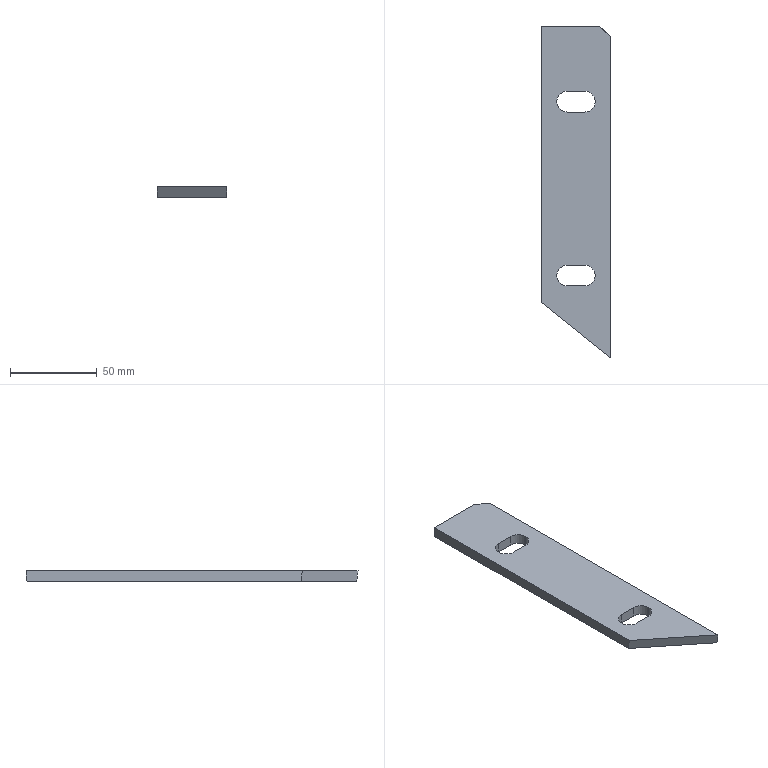Part | STEP file | 粉仓楼梯护栏连接Plate | 1 solid | 17 faces | box 40 x 190.865 x 6 mm | volume 38885 mm3 | plane 11 | cylinder 6 | commonest cylinder face diameters 12 x6
STEP:
#1=CARTESIAN_POINT('',(0.,0.,0.));
#2=DIRECTION('',(0.,0.,1.));
#3=DIRECTION('',(1.,0.,0.));
#4=AXIS2_PLACEMENT_3D('',#1,#2,#3);
#5=CARTESIAN_POINT('',(5.,56.,0.));
#6=VERTEX_POINT('',#5);
#7=CARTESIAN_POINT('',(5.,56.,6.));
#8=VERTEX_POINT('',#7);
#9=CARTESIAN_POINT('',(5.,56.,6.));
#10=DIRECTION('',(0.,0.,1.));
#11=VECTOR('',#10,1.);
#12=LINE('',#9,#11);
#13=CARTESIAN_POINT('',(5.,50.,6.));
#14=DIRECTION('',(0.,0.,1.));
#15=DIRECTION('',(1.,0.,0.));
#16=AXIS2_PLACEMENT_3D('',#13,#14,#15);
#17=CYLINDRICAL_SURFACE('',#16,6.);
#18=CARTESIAN_POINT('',(1.571,0.));
#19=DIRECTION('',(0.,1.));
#20=VECTOR('',#19,1.);
#21=LINE('',#18,#20);
#22=(GEOMETRIC_REPRESENTATION_CONTEXT(2)PARAMETRIC_REPRESENTATION_CONTEXT()REPRESENTATION_CONTEXT('',''));
#23=DEFINITIONAL_REPRESENTATION('',(#21),#22);
#24=PCURVE('',#17,#23);
#25=CARTESIAN_POINT('',(-5.,56.,6.));
#26=DIRECTION('',(0.,1.,0.));
#27=DIRECTION('',(0.,0.,1.));
#28=AXIS2_PLACEMENT_3D('',#25,#26,#27);
#29=PLANE('',#28);
#30=CARTESIAN_POINT('',(0.,10.));
#31=DIRECTION('',(1.,0.));
#32=VECTOR('',#31,1.);
#33=LINE('',#30,#32);
#34=(GEOMETRIC_REPRESENTATION_CONTEXT(2)PARAMETRIC_REPRESENTATION_CONTEXT()REPRESENTATION_CONTEXT('',''));
#35=DEFINITIONAL_REPRESENTATION('',(#33),#34);
#36=PCURVE('',#29,#35);
#37=SURFACE_CURVE('',#12,(#24,#36),.PCURVE_S1.);
#38=EDGE_CURVE('',#6,#8,#37,.T.);
#39=ORIENTED_EDGE('',*,*,#38,.T.);
#40=CARTESIAN_POINT('',(11.,50.,6.));
#41=VERTEX_POINT('',#40);
#42=CARTESIAN_POINT('',(5.,50.,6.));
#43=DIRECTION('',(0.,0.,1.));
#44=DIRECTION('',(1.,0.,0.));
#45=AXIS2_PLACEMENT_3D('',#42,#43,#44);
#46=CIRCLE('',#45,6.);
#47=CARTESIAN_POINT('',(0.,0.));
#48=DIRECTION('',(1.,0.));
#49=VECTOR('',#48,1.);
#50=LINE('',#47,#49);
#51=(GEOMETRIC_REPRESENTATION_CONTEXT(2)PARAMETRIC_REPRESENTATION_CONTEXT()REPRESENTATION_CONTEXT('',''));
#52=DEFINITIONAL_REPRESENTATION('',(#50),#51);
#53=PCURVE('',#17,#52);
#54=CARTESIAN_POINT('',(0.,0.,6.));
#55=DIRECTION('',(0.,0.,1.));
#56=DIRECTION('',(1.,0.,0.));
#57=AXIS2_PLACEMENT_3D('',#54,#55,#56);
#58=PLANE('',#57);
#59=CARTESIAN_POINT('',(5.,50.));
#60=DIRECTION('',(1.,0.));
#61=AXIS2_PLACEMENT_2D('',#59,#60);
#62=CIRCLE('',#61,6.);
#63=(GEOMETRIC_REPRESENTATION_CONTEXT(2)PARAMETRIC_REPRESENTATION_CONTEXT()REPRESENTATION_CONTEXT('',''));
#64=DEFINITIONAL_REPRESENTATION('',(#62),#63);
#65=PCURVE('',#58,#64);
#66=SURFACE_CURVE('',#46,(#53,#65),.PCURVE_S1.);
#67=EDGE_CURVE('',#41,#8,#66,.T.);
#68=ORIENTED_EDGE('',*,*,#67,.F.);
#69=CARTESIAN_POINT('',(11.,50.,0.));
#70=VERTEX_POINT('',#69);
#71=CARTESIAN_POINT('',(11.,50.,6.));
#72=DIRECTION('',(0.,0.,1.));
#73=VECTOR('',#72,1.);
#74=LINE('',#71,#73);
#75=CARTESIAN_POINT('',(0.,0.));
#76=DIRECTION('',(0.,1.));
#77=VECTOR('',#76,1.);
#78=LINE('',#75,#77);
#79=(GEOMETRIC_REPRESENTATION_CONTEXT(2)PARAMETRIC_REPRESENTATION_CONTEXT()REPRESENTATION_CONTEXT('',''));
#80=DEFINITIONAL_REPRESENTATION('',(#78),#79);
#81=PCURVE('',#17,#80);
#82=CARTESIAN_POINT('',(5.,50.,6.));
#83=DIRECTION('',(0.,0.,1.));
#84=DIRECTION('',(1.,0.,0.));
#85=AXIS2_PLACEMENT_3D('',#82,#83,#84);
#86=CYLINDRICAL_SURFACE('',#85,6.);
#87=CARTESIAN_POINT('',(6.283,0.));
#88=DIRECTION('',(0.,1.));
#89=VECTOR('',#88,1.);
#90=LINE('',#87,#89);
#91=(GEOMETRIC_REPRESENTATION_CONTEXT(2)PARAMETRIC_REPRESENTATION_CONTEXT()REPRESENTATION_CONTEXT('',''));
#92=DEFINITIONAL_REPRESENTATION('',(#90),#91);
#93=PCURVE('',#86,#92);
#94=SURFACE_CURVE('',#74,(#81,#93),.PCURVE_S1.);
#95=EDGE_CURVE('',#70,#41,#94,.T.);
#96=ORIENTED_EDGE('',*,*,#95,.F.);
#97=CARTESIAN_POINT('',(5.,50.,0.));
#98=DIRECTION('',(0.,0.,1.));
#99=DIRECTION('',(1.,0.,0.));
#100=AXIS2_PLACEMENT_3D('',#97,#98,#99);
#101=CIRCLE('',#100,6.);
#102=CARTESIAN_POINT('',(0.,-6.));
#103=DIRECTION('',(1.,0.));
#104=VECTOR('',#103,1.);
#105=LINE('',#102,#104);
#106=(GEOMETRIC_REPRESENTATION_CONTEXT(2)PARAMETRIC_REPRESENTATION_CONTEXT()REPRESENTATION_CONTEXT('',''));
#107=DEFINITIONAL_REPRESENTATION('',(#105),#106);
#108=PCURVE('',#17,#107);
#109=CARTESIAN_POINT('',(0.,0.,0.));
#110=DIRECTION('',(0.,0.,1.));
#111=DIRECTION('',(1.,0.,0.));
#112=AXIS2_PLACEMENT_3D('',#109,#110,#111);
#113=PLANE('',#112);
#114=CARTESIAN_POINT('',(5.,50.));
#115=DIRECTION('',(1.,0.));
#116=AXIS2_PLACEMENT_2D('',#114,#115);
#117=CIRCLE('',#116,6.);
#118=(GEOMETRIC_REPRESENTATION_CONTEXT(2)PARAMETRIC_REPRESENTATION_CONTEXT()REPRESENTATION_CONTEXT('',''));
#119=DEFINITIONAL_REPRESENTATION('',(#117),#118);
#120=PCURVE('',#113,#119);
#121=SURFACE_CURVE('',#101,(#108,#120),.PCURVE_S1.);
#122=EDGE_CURVE('',#70,#6,#121,.T.);
#123=ORIENTED_EDGE('',*,*,#122,.T.);
#124=EDGE_LOOP('',(#39,#68,#96,#123));
#125=FACE_BOUND('',#124,.F.);
#126=ADVANCED_FACE('',(#125),#17,.F.);
#127=CARTESIAN_POINT('',(5.,-44.,0.));
#128=VERTEX_POINT('',#127);
#129=CARTESIAN_POINT('',(5.,-44.,6.));
#130=VERTEX_POINT('',#129);
#131=CARTESIAN_POINT('',(5.,-44.,6.));
#132=DIRECTION('',(0.,0.,1.));
#133=VECTOR('',#132,1.);
#134=LINE('',#131,#133);
#135=CARTESIAN_POINT('',(5.,-50.,6.));
#136=DIRECTION('',(0.,0.,1.));
#137=DIRECTION('',(1.,0.,0.));
#138=AXIS2_PLACEMENT_3D('',#135,#136,#137);
#139=CYLINDRICAL_SURFACE('',#138,6.);
#140=CARTESIAN_POINT('',(1.571,0.));
#141=DIRECTION('',(0.,1.));
#142=VECTOR('',#141,1.);
#143=LINE('',#140,#142);
#144=(GEOMETRIC_REPRESENTATION_CONTEXT(2)PARAMETRIC_REPRESENTATION_CONTEXT()REPRESENTATION_CONTEXT('',''));
#145=DEFINITIONAL_REPRESENTATION('',(#143),#144);
#146=PCURVE('',#139,#145);
#147=CARTESIAN_POINT('',(-5.,-44.,6.));
#148=DIRECTION('',(0.,1.,0.));
#149=DIRECTION('',(0.,0.,1.));
#150=AXIS2_PLACEMENT_3D('',#147,#148,#149);
#151=PLANE('',#150);
#152=CARTESIAN_POINT('',(0.,10.));
#153=DIRECTION('',(1.,0.));
#154=VECTOR('',#153,1.);
#155=LINE('',#152,#154);
#156=(GEOMETRIC_REPRESENTATION_CONTEXT(2)PARAMETRIC_REPRESENTATION_CONTEXT()REPRESENTATION_CONTEXT('',''));
#157=DEFINITIONAL_REPRESENTATION('',(#155),#156);
#158=PCURVE('',#151,#157);
#159=SURFACE_CURVE('',#134,(#146,#158),.PCURVE_S1.);
#160=EDGE_CURVE('',#128,#130,#159,.T.);
#161=ORIENTED_EDGE('',*,*,#160,.T.);
#162=CARTESIAN_POINT('',(11.,-50.,6.));
#163=VERTEX_POINT('',#162);
#164=CARTESIAN_POINT('',(5.,-50.,6.));
#165=DIRECTION('',(0.,0.,1.));
#166=DIRECTION('',(1.,0.,0.));
#167=AXIS2_PLACEMENT_3D('',#164,#165,#166);
#168=CIRCLE('',#167,6.);
#169=CARTESIAN_POINT('',(0.,0.));
#170=DIRECTION('',(1.,0.));
#171=VECTOR('',#170,1.);
#172=LINE('',#169,#171);
#173=(GEOMETRIC_REPRESENTATION_CONTEXT(2)PARAMETRIC_REPRESENTATION_CONTEXT()REPRESENTATION_CONTEXT('',''));
#174=DEFINITIONAL_REPRESENTATION('',(#172),#173);
#175=PCURVE('',#139,#174);
#176=CARTESIAN_POINT('',(5.,-50.));
#177=DIRECTION('',(1.,0.));
#178=AXIS2_PLACEMENT_2D('',#176,#177);
#179=CIRCLE('',#178,6.);
#180=(GEOMETRIC_REPRESENTATION_CONTEXT(2)PARAMETRIC_REPRESENTATION_CONTEXT()REPRESENTATION_CONTEXT('',''));
#181=DEFINITIONAL_REPRESENTATION('',(#179),#180);
#182=PCURVE('',#58,#181);
#183=SURFACE_CURVE('',#168,(#175,#182),.PCURVE_S1.);
#184=EDGE_CURVE('',#163,#130,#183,.T.);
#185=ORIENTED_EDGE('',*,*,#184,.F.);
#186=CARTESIAN_POINT('',(11.,-50.,0.));
#187=VERTEX_POINT('',#186);
#188=CARTESIAN_POINT('',(11.,-50.,6.));
#189=DIRECTION('',(0.,0.,1.));
#190=VECTOR('',#189,1.);
#191=LINE('',#188,#190);
#192=CARTESIAN_POINT('',(0.,0.));
#193=DIRECTION('',(0.,1.));
#194=VECTOR('',#193,1.);
#195=LINE('',#192,#194);
#196=(GEOMETRIC_REPRESENTATION_CONTEXT(2)PARAMETRIC_REPRESENTATION_CONTEXT()REPRESENTATION_CONTEXT('',''));
#197=DEFINITIONAL_REPRESENTATION('',(#195),#196);
#198=PCURVE('',#139,#197);
#199=CARTESIAN_POINT('',(5.,-50.,6.));
#200=DIRECTION('',(0.,0.,1.));
#201=DIRECTION('',(1.,0.,0.));
#202=AXIS2_PLACEMENT_3D('',#199,#200,#201);
#203=CYLINDRICAL_SURFACE('',#202,6.);
#204=CARTESIAN_POINT('',(6.283,0.));
#205=DIRECTION('',(0.,1.));
#206=VECTOR('',#205,1.);
#207=LINE('',#204,#206);
#208=(GEOMETRIC_REPRESENTATION_CONTEXT(2)PARAMETRIC_REPRESENTATION_CONTEXT()REPRESENTATION_CONTEXT('',''));
#209=DEFINITIONAL_REPRESENTATION('',(#207),#208);
#210=PCURVE('',#203,#209);
#211=SURFACE_CURVE('',#191,(#198,#210),.PCURVE_S1.);
#212=EDGE_CURVE('',#187,#163,#211,.T.);
#213=ORIENTED_EDGE('',*,*,#212,.F.);
#214=CARTESIAN_POINT('',(5.,-50.,0.));
#215=DIRECTION('',(0.,0.,1.));
#216=DIRECTION('',(1.,0.,0.));
#217=AXIS2_PLACEMENT_3D('',#214,#215,#216);
#218=CIRCLE('',#217,6.);
#219=CARTESIAN_POINT('',(0.,-6.));
#220=DIRECTION('',(1.,0.));
#221=VECTOR('',#220,1.);
#222=LINE('',#219,#221);
#223=(GEOMETRIC_REPRESENTATION_CONTEXT(2)PARAMETRIC_REPRESENTATION_CONTEXT()REPRESENTATION_CONTEXT('',''));
#224=DEFINITIONAL_REPRESENTATION('',(#222),#223);
#225=PCURVE('',#139,#224);
#226=CARTESIAN_POINT('',(5.,-50.));
#227=DIRECTION('',(1.,0.));
#228=AXIS2_PLACEMENT_2D('',#226,#227);
#229=CIRCLE('',#228,6.);
#230=(GEOMETRIC_REPRESENTATION_CONTEXT(2)PARAMETRIC_REPRESENTATION_CONTEXT()REPRESENTATION_CONTEXT('',''));
#231=DEFINITIONAL_REPRESENTATION('',(#229),#230);
#232=PCURVE('',#113,#231);
#233=SURFACE_CURVE('',#218,(#225,#232),.PCURVE_S1.);
#234=EDGE_CURVE('',#187,#128,#233,.T.);
#235=ORIENTED_EDGE('',*,*,#234,.T.);
#236=EDGE_LOOP('',(#161,#185,#213,#235));
#237=FACE_BOUND('',#236,.F.);
#238=ADVANCED_FACE('',(#237),#139,.F.);
#239=CARTESIAN_POINT('',(20.,-96.589,0.));
#240=VERTEX_POINT('',#239);
#241=CARTESIAN_POINT('',(20.,87.469,0.));
#242=VERTEX_POINT('',#241);
#243=CARTESIAN_POINT('',(20.,92.,0.));
#244=DIRECTION('',(0.,1.,0.));
#245=VECTOR('',#244,1.);
#246=LINE('',#243,#245);
#247=CARTESIAN_POINT('',(20.,92.,6.));
#248=DIRECTION('',(-1.,0.,0.));
#249=DIRECTION('',(0.,-1.,0.));
#250=AXIS2_PLACEMENT_3D('',#247,#248,#249);
#251=PLANE('',#250);
#252=CARTESIAN_POINT('',(0.,-6.));
#253=DIRECTION('',(-1.,0.));
#254=VECTOR('',#253,1.);
#255=LINE('',#252,#254);
#256=(GEOMETRIC_REPRESENTATION_CONTEXT(2)PARAMETRIC_REPRESENTATION_CONTEXT()REPRESENTATION_CONTEXT('',''));
#257=DEFINITIONAL_REPRESENTATION('',(#255),#256);
#258=PCURVE('',#251,#257);
#259=CARTESIAN_POINT('',(20.,92.));
#260=DIRECTION('',(0.,1.));
#261=VECTOR('',#260,1.);
#262=LINE('',#259,#261);
#263=(GEOMETRIC_REPRESENTATION_CONTEXT(2)PARAMETRIC_REPRESENTATION_CONTEXT()REPRESENTATION_CONTEXT('',''));
#264=DEFINITIONAL_REPRESENTATION('',(#262),#263);
#265=PCURVE('',#113,#264);
#266=SURFACE_CURVE('',#246,(#258,#265),.PCURVE_S1.);
#267=EDGE_CURVE('',#240,#242,#266,.T.);
#268=ORIENTED_EDGE('',*,*,#267,.T.);
#269=CARTESIAN_POINT('',(20.,87.469,6.));
#270=VERTEX_POINT('',#269);
#271=CARTESIAN_POINT('',(20.,87.469,0.));
#272=DIRECTION('',(0.,0.,1.));
#273=VECTOR('',#272,1.);
#274=LINE('',#271,#273);
#275=CARTESIAN_POINT('',(4.531,-6.));
#276=DIRECTION('',(0.,1.));
#277=VECTOR('',#276,1.);
#278=LINE('',#275,#277);
#279=(GEOMETRIC_REPRESENTATION_CONTEXT(2)PARAMETRIC_REPRESENTATION_CONTEXT()REPRESENTATION_CONTEXT('',''));
#280=DEFINITIONAL_REPRESENTATION('',(#278),#279);
#281=PCURVE('',#251,#280);
#282=CARTESIAN_POINT('',(20.,87.469,0.));
#283=DIRECTION('',(-0.6508,-0.7593,0.));
#284=DIRECTION('',(0.7593,-0.6508,0.));
#285=AXIS2_PLACEMENT_3D('',#282,#283,#284);
#286=PLANE('',#285);
#287=CARTESIAN_POINT('',(0.,0.));
#288=DIRECTION('',(0.,1.));
#289=VECTOR('',#288,1.);
#290=LINE('',#287,#289);
#291=(GEOMETRIC_REPRESENTATION_CONTEXT(2)PARAMETRIC_REPRESENTATION_CONTEXT()REPRESENTATION_CONTEXT('',''));
#292=DEFINITIONAL_REPRESENTATION('',(#290),#291);
#293=PCURVE('',#286,#292);
#294=SURFACE_CURVE('',#274,(#281,#293),.PCURVE_S1.);
#295=EDGE_CURVE('',#242,#270,#294,.T.);
#296=ORIENTED_EDGE('',*,*,#295,.T.);
#297=CARTESIAN_POINT('',(20.,-97.396,6.));
#298=VERTEX_POINT('',#297);
#299=CARTESIAN_POINT('',(20.,92.,6.));
#300=DIRECTION('',(0.,1.,0.));
#301=VECTOR('',#300,1.);
#302=LINE('',#299,#301);
#303=CARTESIAN_POINT('',(0.,0.));
#304=DIRECTION('',(-1.,0.));
#305=VECTOR('',#304,1.);
#306=LINE('',#303,#305);
#307=(GEOMETRIC_REPRESENTATION_CONTEXT(2)PARAMETRIC_REPRESENTATION_CONTEXT()REPRESENTATION_CONTEXT('',''));
#308=DEFINITIONAL_REPRESENTATION('',(#306),#307);
#309=PCURVE('',#251,#308);
#310=CARTESIAN_POINT('',(20.,92.));
#311=DIRECTION('',(0.,1.));
#312=VECTOR('',#311,1.);
#313=LINE('',#310,#312);
#314=(GEOMETRIC_REPRESENTATION_CONTEXT(2)PARAMETRIC_REPRESENTATION_CONTEXT()REPRESENTATION_CONTEXT('',''));
#315=DEFINITIONAL_REPRESENTATION('',(#313),#314);
#316=PCURVE('',#58,#315);
#317=SURFACE_CURVE('',#302,(#309,#316),.PCURVE_S1.);
#318=EDGE_CURVE('',#298,#270,#317,.T.);
#319=ORIENTED_EDGE('',*,*,#318,.F.);
#320=CARTESIAN_POINT('',(20.,-97.134,4.055));
#321=DIRECTION('',(0.,-0.1334,0.9911));
#322=VECTOR('',#321,1.);
#323=LINE('',#320,#322);
#324=CARTESIAN_POINT('',(189.134,-1.945));
#325=DIRECTION('',(0.1334,0.9911));
#326=VECTOR('',#325,1.);
#327=LINE('',#324,#326);
#328=(GEOMETRIC_REPRESENTATION_CONTEXT(2)PARAMETRIC_REPRESENTATION_CONTEXT()REPRESENTATION_CONTEXT('',''));
#329=DEFINITIONAL_REPRESENTATION('',(#327),#328);
#330=PCURVE('',#251,#329);
#331=CARTESIAN_POINT('',(2925.063,-2415.047,-41.545));
#332=DIRECTION('',(-0.6213,-0.7766,-0.1045));
#333=DIRECTION('',(0.7809,-0.6247,0.));
#334=AXIS2_PLACEMENT_3D('',#331,#332,#333);
#335=PLANE('',#334);
#336=CARTESIAN_POINT('',(-3716.461,45.851));
#337=DIRECTION('',(0.08333,0.9965));
#338=VECTOR('',#337,1.);
#339=LINE('',#336,#338);
#340=(GEOMETRIC_REPRESENTATION_CONTEXT(2)PARAMETRIC_REPRESENTATION_CONTEXT()REPRESENTATION_CONTEXT('',''));
#341=DEFINITIONAL_REPRESENTATION('',(#339),#340);
#342=PCURVE('',#335,#341);
#343=SURFACE_CURVE('',#323,(#330,#342),.PCURVE_S1.);
#344=EDGE_CURVE('',#240,#298,#343,.T.);
#345=ORIENTED_EDGE('',*,*,#344,.F.);
#346=EDGE_LOOP('',(#268,#296,#319,#345));
#347=FACE_BOUND('',#346,.T.);
#348=ADVANCED_FACE('',(#347),#251,.F.);
#349=CARTESIAN_POINT('',(-20.,92.839,0.));
#350=VERTEX_POINT('',#349);
#351=CARTESIAN_POINT('',(-20.,-64.589,0.));
#352=VERTEX_POINT('',#351);
#353=CARTESIAN_POINT('',(-20.,92.,0.));
#354=DIRECTION('',(0.,-1.,0.));
#355=VECTOR('',#354,1.);
#356=LINE('',#353,#355);
#357=CARTESIAN_POINT('',(-20.,92.,6.));
#358=DIRECTION('',(1.,0.,0.));
#359=DIRECTION('',(0.,1.,0.));
#360=AXIS2_PLACEMENT_3D('',#357,#358,#359);
#361=PLANE('',#360);
#362=CARTESIAN_POINT('',(0.,-6.));
#363=DIRECTION('',(-1.,0.));
#364=VECTOR('',#363,1.);
#365=LINE('',#362,#364);
#366=(GEOMETRIC_REPRESENTATION_CONTEXT(2)PARAMETRIC_REPRESENTATION_CONTEXT()REPRESENTATION_CONTEXT('',''));
#367=DEFINITIONAL_REPRESENTATION('',(#365),#366);
#368=PCURVE('',#361,#367);
#369=CARTESIAN_POINT('',(-20.,92.));
#370=DIRECTION('',(0.,-1.));
#371=VECTOR('',#370,1.);
#372=LINE('',#369,#371);
#373=(GEOMETRIC_REPRESENTATION_CONTEXT(2)PARAMETRIC_REPRESENTATION_CONTEXT()REPRESENTATION_CONTEXT('',''));
#374=DEFINITIONAL_REPRESENTATION('',(#372),#373);
#375=PCURVE('',#113,#374);
#376=SURFACE_CURVE('',#356,(#368,#375),.PCURVE_S1.);
#377=EDGE_CURVE('',#350,#352,#376,.T.);
#378=ORIENTED_EDGE('',*,*,#377,.T.);
#379=CARTESIAN_POINT('',(-20.,-65.396,6.));
#380=VERTEX_POINT('',#379);
#381=CARTESIAN_POINT('',(-20.,-66.497,14.178));
#382=DIRECTION('',(0.,0.1334,-0.9911));
#383=VECTOR('',#382,1.);
#384=LINE('',#381,#383);
#385=CARTESIAN_POINT('',(-158.497,8.178));
#386=DIRECTION('',(0.1334,-0.9911));
#387=VECTOR('',#386,1.);
#388=LINE('',#385,#387);
#389=(GEOMETRIC_REPRESENTATION_CONTEXT(2)PARAMETRIC_REPRESENTATION_CONTEXT()REPRESENTATION_CONTEXT('',''));
#390=DEFINITIONAL_REPRESENTATION('',(#388),#389);
#391=PCURVE('',#361,#390);
#392=CARTESIAN_POINT('',(-3766.835,56.031));
#393=DIRECTION('',(-0.08333,-0.9965));
#394=VECTOR('',#393,1.);
#395=LINE('',#392,#394);
#396=(GEOMETRIC_REPRESENTATION_CONTEXT(2)PARAMETRIC_REPRESENTATION_CONTEXT()REPRESENTATION_CONTEXT('',''));
#397=DEFINITIONAL_REPRESENTATION('',(#395),#396);
#398=PCURVE('',#335,#397);
#399=SURFACE_CURVE('',#384,(#391,#398),.PCURVE_S1.);
#400=EDGE_CURVE('',#380,#352,#399,.T.);
#401=ORIENTED_EDGE('',*,*,#400,.F.);
#402=CARTESIAN_POINT('',(-20.,93.469,6.));
#403=VERTEX_POINT('',#402);
#404=CARTESIAN_POINT('',(-20.,92.,6.));
#405=DIRECTION('',(0.,-1.,0.));
#406=VECTOR('',#405,1.);
#407=LINE('',#404,#406);
#408=CARTESIAN_POINT('',(0.,0.));
#409=DIRECTION('',(-1.,0.));
#410=VECTOR('',#409,1.);
#411=LINE('',#408,#410);
#412=(GEOMETRIC_REPRESENTATION_CONTEXT(2)PARAMETRIC_REPRESENTATION_CONTEXT()REPRESENTATION_CONTEXT('',''));
#413=DEFINITIONAL_REPRESENTATION('',(#411),#412);
#414=PCURVE('',#361,#413);
#415=CARTESIAN_POINT('',(-20.,92.));
#416=DIRECTION('',(0.,-1.));
#417=VECTOR('',#416,1.);
#418=LINE('',#415,#417);
#419=(GEOMETRIC_REPRESENTATION_CONTEXT(2)PARAMETRIC_REPRESENTATION_CONTEXT()REPRESENTATION_CONTEXT('',''));
#420=DEFINITIONAL_REPRESENTATION('',(#418),#419);
#421=PCURVE('',#58,#420);
#422=SURFACE_CURVE('',#407,(#414,#421),.PCURVE_S1.);
#423=EDGE_CURVE('',#403,#380,#422,.T.);
#424=ORIENTED_EDGE('',*,*,#423,.F.);
#425=CARTESIAN_POINT('',(-20.,93.285,4.249));
#426=DIRECTION('',(0.,0.1045,0.9945));
#427=VECTOR('',#426,1.);
#428=LINE('',#425,#427);
#429=CARTESIAN_POINT('',(1.285,-1.751));
#430=DIRECTION('',(0.1045,0.9945));
#431=VECTOR('',#430,1.);
#432=LINE('',#429,#431);
#433=(GEOMETRIC_REPRESENTATION_CONTEXT(2)PARAMETRIC_REPRESENTATION_CONTEXT()REPRESENTATION_CONTEXT('',''));
#434=DEFINITIONAL_REPRESENTATION('',(#432),#433);
#435=PCURVE('',#361,#434);
#436=CARTESIAN_POINT('',(17.5,88.472,-41.545));
#437=DIRECTION('',(0.,0.9945,-0.1045));
#438=DIRECTION('',(0.,-0.1045,-0.9945));
#439=AXIS2_PLACEMENT_3D('',#436,#437,#438);
#440=PLANE('',#439);
#441=CARTESIAN_POINT('',(-46.047,37.5));
#442=DIRECTION('',(-1.,0.));
#443=VECTOR('',#442,1.);
#444=LINE('',#441,#443);
#445=(GEOMETRIC_REPRESENTATION_CONTEXT(2)PARAMETRIC_REPRESENTATION_CONTEXT()REPRESENTATION_CONTEXT('',''));
#446=DEFINITIONAL_REPRESENTATION('',(#444),#445);
#447=PCURVE('',#440,#446);
#448=SURFACE_CURVE('',#428,(#435,#447),.PCURVE_S1.);
#449=EDGE_CURVE('',#350,#403,#448,.T.);
#450=ORIENTED_EDGE('',*,*,#449,.F.);
#451=EDGE_LOOP('',(#378,#401,#424,#450));
#452=FACE_BOUND('',#451,.T.);
#453=ADVANCED_FACE('',(#452),#361,.F.);
#454=CARTESIAN_POINT('',(13.,93.469,6.));
#455=VERTEX_POINT('',#454);
#456=CARTESIAN_POINT('',(20.,87.469,6.));
#457=DIRECTION('',(0.7593,-0.6508,0.));
#458=VECTOR('',#457,1.);
#459=LINE('',#456,#458);
#460=CARTESIAN_POINT('',(20.,87.469));
#461=DIRECTION('',(0.7593,-0.6508));
#462=VECTOR('',#461,1.);
#463=LINE('',#460,#462);
#464=(GEOMETRIC_REPRESENTATION_CONTEXT(2)PARAMETRIC_REPRESENTATION_CONTEXT()REPRESENTATION_CONTEXT('',''));
#465=DEFINITIONAL_REPRESENTATION('',(#463),#464);
#466=PCURVE('',#58,#465);
#467=CARTESIAN_POINT('',(0.,6.));
#468=DIRECTION('',(1.,0.));
#469=VECTOR('',#468,1.);
#470=LINE('',#467,#469);
#471=(GEOMETRIC_REPRESENTATION_CONTEXT(2)PARAMETRIC_REPRESENTATION_CONTEXT()REPRESENTATION_CONTEXT('',''));
#472=DEFINITIONAL_REPRESENTATION('',(#470),#471);
#473=PCURVE('',#286,#472);
#474=SURFACE_CURVE('',#459,(#466,#473),.PCURVE_S1.);
#475=EDGE_CURVE('',#455,#270,#474,.T.);
#476=ORIENTED_EDGE('',*,*,#475,.F.);
#477=CARTESIAN_POINT('',(-20.,93.469,6.));
#478=DIRECTION('',(1.,0.,0.));
#479=VECTOR('',#478,1.);
#480=LINE('',#477,#479);
#481=CARTESIAN_POINT('',(-20.,93.469));
#482=DIRECTION('',(1.,0.));
#483=VECTOR('',#482,1.);
#484=LINE('',#481,#483);
#485=(GEOMETRIC_REPRESENTATION_CONTEXT(2)PARAMETRIC_REPRESENTATION_CONTEXT()REPRESENTATION_CONTEXT('',''));
#486=DEFINITIONAL_REPRESENTATION('',(#484),#485);
#487=PCURVE('',#58,#486);
#488=CARTESIAN_POINT('',(-47.807,37.5));
#489=DIRECTION('',(0.,-1.));
#490=VECTOR('',#489,1.);
#491=LINE('',#488,#490);
#492=(GEOMETRIC_REPRESENTATION_CONTEXT(2)PARAMETRIC_REPRESENTATION_CONTEXT()REPRESENTATION_CONTEXT('',''));
#493=DEFINITIONAL_REPRESENTATION('',(#491),#492);
#494=PCURVE('',#440,#493);
#495=SURFACE_CURVE('',#480,(#487,#494),.PCURVE_S1.);
#496=EDGE_CURVE('',#403,#455,#495,.T.);
#497=ORIENTED_EDGE('',*,*,#496,.F.);
#498=ORIENTED_EDGE('',*,*,#423,.T.);
#499=CARTESIAN_POINT('',(34.567,-109.049,6.));
#500=DIRECTION('',(-0.7809,0.6247,0.));
#501=VECTOR('',#500,1.);
#502=LINE('',#499,#501);
#503=CARTESIAN_POINT('',(34.567,-109.049));
#504=DIRECTION('',(-0.7809,0.6247));
#505=VECTOR('',#504,1.);
#506=LINE('',#503,#505);
#507=(GEOMETRIC_REPRESENTATION_CONTEXT(2)PARAMETRIC_REPRESENTATION_CONTEXT()REPRESENTATION_CONTEXT('',''));
#508=DEFINITIONAL_REPRESENTATION('',(#506),#507);
#509=PCURVE('',#58,#508);
#510=CARTESIAN_POINT('',(-3697.643,47.807));
#511=DIRECTION('',(-1.,0.));
#512=VECTOR('',#511,1.);
#513=LINE('',#510,#512);
#514=(GEOMETRIC_REPRESENTATION_CONTEXT(2)PARAMETRIC_REPRESENTATION_CONTEXT()REPRESENTATION_CONTEXT('',''));
#515=DEFINITIONAL_REPRESENTATION('',(#513),#514);
#516=PCURVE('',#335,#515);
#517=SURFACE_CURVE('',#502,(#509,#516),.PCURVE_S1.);
#518=EDGE_CURVE('',#298,#380,#517,.T.);
#519=ORIENTED_EDGE('',*,*,#518,.F.);
#520=ORIENTED_EDGE('',*,*,#318,.T.);
#521=EDGE_LOOP('',(#476,#497,#498,#519,#520));
#522=FACE_BOUND('',#521,.T.);
#523=CARTESIAN_POINT('',(-5.,44.,6.));
#524=VERTEX_POINT('',#523);
#525=CARTESIAN_POINT('',(5.,44.,6.));
#526=VERTEX_POINT('',#525);
#527=CARTESIAN_POINT('',(-5.,44.,6.));
#528=DIRECTION('',(1.,0.,0.));
#529=VECTOR('',#528,1.);
#530=LINE('',#527,#529);
#531=CARTESIAN_POINT('',(-5.,44.));
#532=DIRECTION('',(1.,0.));
#533=VECTOR('',#532,1.);
#534=LINE('',#531,#533);
#535=(GEOMETRIC_REPRESENTATION_CONTEXT(2)PARAMETRIC_REPRESENTATION_CONTEXT()REPRESENTATION_CONTEXT('',''));
#536=DEFINITIONAL_REPRESENTATION('',(#534),#535);
#537=PCURVE('',#58,#536);
#538=CARTESIAN_POINT('',(-5.,44.,6.));
#539=DIRECTION('',(0.,-1.,0.));
#540=DIRECTION('',(0.,0.,-1.));
#541=AXIS2_PLACEMENT_3D('',#538,#539,#540);
#542=PLANE('',#541);
#543=CARTESIAN_POINT('',(0.,0.));
#544=DIRECTION('',(0.,1.));
#545=VECTOR('',#544,1.);
#546=LINE('',#543,#545);
#547=(GEOMETRIC_REPRESENTATION_CONTEXT(2)PARAMETRIC_REPRESENTATION_CONTEXT()REPRESENTATION_CONTEXT('',''));
#548=DEFINITIONAL_REPRESENTATION('',(#546),#547);
#549=PCURVE('',#542,#548);
#550=SURFACE_CURVE('',#530,(#537,#549),.PCURVE_S1.);
#551=EDGE_CURVE('',#524,#526,#550,.T.);
#552=ORIENTED_EDGE('',*,*,#551,.F.);
#553=CARTESIAN_POINT('',(-5.,56.,6.));
#554=VERTEX_POINT('',#553);
#555=CARTESIAN_POINT('',(-5.,50.,6.));
#556=DIRECTION('',(0.,0.,1.));
#557=DIRECTION('',(1.,0.,0.));
#558=AXIS2_PLACEMENT_3D('',#555,#556,#557);
#559=CIRCLE('',#558,6.);
#560=CARTESIAN_POINT('',(-5.,50.));
#561=DIRECTION('',(1.,0.));
#562=AXIS2_PLACEMENT_2D('',#560,#561);
#563=CIRCLE('',#562,6.);
#564=(GEOMETRIC_REPRESENTATION_CONTEXT(2)PARAMETRIC_REPRESENTATION_CONTEXT()REPRESENTATION_CONTEXT('',''));
#565=DEFINITIONAL_REPRESENTATION('',(#563),#564);
#566=PCURVE('',#58,#565);
#567=CARTESIAN_POINT('',(-5.,50.,6.));
#568=DIRECTION('',(0.,0.,1.));
#569=DIRECTION('',(1.,0.,0.));
#570=AXIS2_PLACEMENT_3D('',#567,#568,#569);
#571=CYLINDRICAL_SURFACE('',#570,6.);
#572=CARTESIAN_POINT('',(0.,0.));
#573=DIRECTION('',(1.,0.));
#574=VECTOR('',#573,1.);
#575=LINE('',#572,#574);
#576=(GEOMETRIC_REPRESENTATION_CONTEXT(2)PARAMETRIC_REPRESENTATION_CONTEXT()REPRESENTATION_CONTEXT('',''));
#577=DEFINITIONAL_REPRESENTATION('',(#575),#576);
#578=PCURVE('',#571,#577);
#579=SURFACE_CURVE('',#559,(#566,#578),.PCURVE_S1.);
#580=EDGE_CURVE('',#554,#524,#579,.T.);
#581=ORIENTED_EDGE('',*,*,#580,.F.);
#582=CARTESIAN_POINT('',(-5.,56.,6.));
#583=DIRECTION('',(1.,0.,0.));
#584=VECTOR('',#583,1.);
#585=LINE('',#582,#584);
#586=CARTESIAN_POINT('',(-5.,56.));
#587=DIRECTION('',(1.,0.));
#588=VECTOR('',#587,1.);
#589=LINE('',#586,#588);
#590=(GEOMETRIC_REPRESENTATION_CONTEXT(2)PARAMETRIC_REPRESENTATION_CONTEXT()REPRESENTATION_CONTEXT('',''));
#591=DEFINITIONAL_REPRESENTATION('',(#589),#590);
#592=PCURVE('',#58,#591);
#593=CARTESIAN_POINT('',(0.,0.));
#594=DIRECTION('',(0.,1.));
#595=VECTOR('',#594,1.);
#596=LINE('',#593,#595);
#597=(GEOMETRIC_REPRESENTATION_CONTEXT(2)PARAMETRIC_REPRESENTATION_CONTEXT()REPRESENTATION_CONTEXT('',''));
#598=DEFINITIONAL_REPRESENTATION('',(#596),#597);
#599=PCURVE('',#29,#598);
#600=SURFACE_CURVE('',#585,(#592,#599),.PCURVE_S1.);
#601=EDGE_CURVE('',#554,#8,#600,.T.);
#602=ORIENTED_EDGE('',*,*,#601,.T.);
#603=ORIENTED_EDGE('',*,*,#67,.F.);
#604=CARTESIAN_POINT('',(5.,50.,6.));
#605=DIRECTION('',(0.,0.,1.));
#606=DIRECTION('',(1.,0.,0.));
#607=AXIS2_PLACEMENT_3D('',#604,#605,#606);
#608=CIRCLE('',#607,6.);
#609=CARTESIAN_POINT('',(5.,50.));
#610=DIRECTION('',(1.,0.));
#611=AXIS2_PLACEMENT_2D('',#609,#610);
#612=CIRCLE('',#611,6.);
#613=(GEOMETRIC_REPRESENTATION_CONTEXT(2)PARAMETRIC_REPRESENTATION_CONTEXT()REPRESENTATION_CONTEXT('',''));
#614=DEFINITIONAL_REPRESENTATION('',(#612),#613);
#615=PCURVE('',#58,#614);
#616=CARTESIAN_POINT('',(0.,0.));
#617=DIRECTION('',(1.,0.));
#618=VECTOR('',#617,1.);
#619=LINE('',#616,#618);
#620=(GEOMETRIC_REPRESENTATION_CONTEXT(2)PARAMETRIC_REPRESENTATION_CONTEXT()REPRESENTATION_CONTEXT('',''));
#621=DEFINITIONAL_REPRESENTATION('',(#619),#620);
#622=PCURVE('',#86,#621);
#623=SURFACE_CURVE('',#608,(#615,#622),.PCURVE_S1.);
#624=EDGE_CURVE('',#526,#41,#623,.T.);
#625=ORIENTED_EDGE('',*,*,#624,.F.);
#626=EDGE_LOOP('',(#552,#581,#602,#603,#625));
#627=FACE_BOUND('',#626,.T.);
#628=CARTESIAN_POINT('',(-5.,-56.,6.));
#629=VERTEX_POINT('',#628);
#630=CARTESIAN_POINT('',(5.,-56.,6.));
#631=VERTEX_POINT('',#630);
#632=CARTESIAN_POINT('',(-5.,-56.,6.));
#633=DIRECTION('',(1.,0.,0.));
#634=VECTOR('',#633,1.);
#635=LINE('',#632,#634);
#636=CARTESIAN_POINT('',(-5.,-56.));
#637=DIRECTION('',(1.,0.));
#638=VECTOR('',#637,1.);
#639=LINE('',#636,#638);
#640=(GEOMETRIC_REPRESENTATION_CONTEXT(2)PARAMETRIC_REPRESENTATION_CONTEXT()REPRESENTATION_CONTEXT('',''));
#641=DEFINITIONAL_REPRESENTATION('',(#639),#640);
#642=PCURVE('',#58,#641);
#643=CARTESIAN_POINT('',(-5.,-56.,6.));
#644=DIRECTION('',(0.,-1.,0.));
#645=DIRECTION('',(0.,0.,-1.));
#646=AXIS2_PLACEMENT_3D('',#643,#644,#645);
#647=PLANE('',#646);
#648=CARTESIAN_POINT('',(0.,0.));
#649=DIRECTION('',(0.,1.));
#650=VECTOR('',#649,1.);
#651=LINE('',#648,#650);
#652=(GEOMETRIC_REPRESENTATION_CONTEXT(2)PARAMETRIC_REPRESENTATION_CONTEXT()REPRESENTATION_CONTEXT('',''));
#653=DEFINITIONAL_REPRESENTATION('',(#651),#652);
#654=PCURVE('',#647,#653);
#655=SURFACE_CURVE('',#635,(#642,#654),.PCURVE_S1.);
#656=EDGE_CURVE('',#629,#631,#655,.T.);
#657=ORIENTED_EDGE('',*,*,#656,.F.);
#658=CARTESIAN_POINT('',(-5.,-44.,6.));
#659=VERTEX_POINT('',#658);
#660=CARTESIAN_POINT('',(-5.,-50.,6.));
#661=DIRECTION('',(0.,0.,1.));
#662=DIRECTION('',(1.,0.,0.));
#663=AXIS2_PLACEMENT_3D('',#660,#661,#662);
#664=CIRCLE('',#663,6.);
#665=CARTESIAN_POINT('',(-5.,-50.));
#666=DIRECTION('',(1.,0.));
#667=AXIS2_PLACEMENT_2D('',#665,#666);
#668=CIRCLE('',#667,6.);
#669=(GEOMETRIC_REPRESENTATION_CONTEXT(2)PARAMETRIC_REPRESENTATION_CONTEXT()REPRESENTATION_CONTEXT('',''));
#670=DEFINITIONAL_REPRESENTATION('',(#668),#669);
#671=PCURVE('',#58,#670);
#672=CARTESIAN_POINT('',(-5.,-50.,6.));
#673=DIRECTION('',(0.,0.,1.));
#674=DIRECTION('',(1.,0.,0.));
#675=AXIS2_PLACEMENT_3D('',#672,#673,#674);
#676=CYLINDRICAL_SURFACE('',#675,6.);
#677=CARTESIAN_POINT('',(0.,0.));
#678=DIRECTION('',(1.,0.));
#679=VECTOR('',#678,1.);
#680=LINE('',#677,#679);
#681=(GEOMETRIC_REPRESENTATION_CONTEXT(2)PARAMETRIC_REPRESENTATION_CONTEXT()REPRESENTATION_CONTEXT('',''));
#682=DEFINITIONAL_REPRESENTATION('',(#680),#681);
#683=PCURVE('',#676,#682);
#684=SURFACE_CURVE('',#664,(#671,#683),.PCURVE_S1.);
#685=EDGE_CURVE('',#659,#629,#684,.T.);
#686=ORIENTED_EDGE('',*,*,#685,.F.);
#687=CARTESIAN_POINT('',(-5.,-44.,6.));
#688=DIRECTION('',(1.,0.,0.));
#689=VECTOR('',#688,1.);
#690=LINE('',#687,#689);
#691=CARTESIAN_POINT('',(-5.,-44.));
#692=DIRECTION('',(1.,0.));
#693=VECTOR('',#692,1.);
#694=LINE('',#691,#693);
#695=(GEOMETRIC_REPRESENTATION_CONTEXT(2)PARAMETRIC_REPRESENTATION_CONTEXT()REPRESENTATION_CONTEXT('',''));
#696=DEFINITIONAL_REPRESENTATION('',(#694),#695);
#697=PCURVE('',#58,#696);
#698=CARTESIAN_POINT('',(0.,0.));
#699=DIRECTION('',(0.,1.));
#700=VECTOR('',#699,1.);
#701=LINE('',#698,#700);
#702=(GEOMETRIC_REPRESENTATION_CONTEXT(2)PARAMETRIC_REPRESENTATION_CONTEXT()REPRESENTATION_CONTEXT('',''));
#703=DEFINITIONAL_REPRESENTATION('',(#701),#702);
#704=PCURVE('',#151,#703);
#705=SURFACE_CURVE('',#690,(#697,#704),.PCURVE_S1.);
#706=EDGE_CURVE('',#659,#130,#705,.T.);
#707=ORIENTED_EDGE('',*,*,#706,.T.);
#708=ORIENTED_EDGE('',*,*,#184,.F.);
#709=CARTESIAN_POINT('',(5.,-50.,6.));
#710=DIRECTION('',(0.,0.,1.));
#711=DIRECTION('',(1.,0.,0.));
#712=AXIS2_PLACEMENT_3D('',#709,#710,#711);
#713=CIRCLE('',#712,6.);
#714=CARTESIAN_POINT('',(5.,-50.));
#715=DIRECTION('',(1.,0.));
#716=AXIS2_PLACEMENT_2D('',#714,#715);
#717=CIRCLE('',#716,6.);
#718=(GEOMETRIC_REPRESENTATION_CONTEXT(2)PARAMETRIC_REPRESENTATION_CONTEXT()REPRESENTATION_CONTEXT('',''));
#719=DEFINITIONAL_REPRESENTATION('',(#717),#718);
#720=PCURVE('',#58,#719);
#721=CARTESIAN_POINT('',(0.,0.));
#722=DIRECTION('',(1.,0.));
#723=VECTOR('',#722,1.);
#724=LINE('',#721,#723);
#725=(GEOMETRIC_REPRESENTATION_CONTEXT(2)PARAMETRIC_REPRESENTATION_CONTEXT()REPRESENTATION_CONTEXT('',''));
#726=DEFINITIONAL_REPRESENTATION('',(#724),#725);
#727=PCURVE('',#203,#726);
#728=SURFACE_CURVE('',#713,(#720,#727),.PCURVE_S1.);
#729=EDGE_CURVE('',#631,#163,#728,.T.);
#730=ORIENTED_EDGE('',*,*,#729,.F.);
#731=EDGE_LOOP('',(#657,#686,#707,#708,#730));
#732=FACE_BOUND('',#731,.T.);
#733=ADVANCED_FACE('',(#522,#627,#732),#58,.T.);
#734=CARTESIAN_POINT('',(-5.,56.,0.));
#735=VERTEX_POINT('',#734);
#736=CARTESIAN_POINT('',(-5.,56.,0.));
#737=DIRECTION('',(1.,0.,0.));
#738=VECTOR('',#737,1.);
#739=LINE('',#736,#738);
#740=CARTESIAN_POINT('',(-5.,56.));
#741=DIRECTION('',(1.,0.));
#742=VECTOR('',#741,1.);
#743=LINE('',#740,#742);
#744=(GEOMETRIC_REPRESENTATION_CONTEXT(2)PARAMETRIC_REPRESENTATION_CONTEXT()REPRESENTATION_CONTEXT('',''));
#745=DEFINITIONAL_REPRESENTATION('',(#743),#744);
#746=PCURVE('',#113,#745);
#747=CARTESIAN_POINT('',(-6.,0.));
#748=DIRECTION('',(0.,1.));
#749=VECTOR('',#748,1.);
#750=LINE('',#747,#749);
#751=(GEOMETRIC_REPRESENTATION_CONTEXT(2)PARAMETRIC_REPRESENTATION_CONTEXT()REPRESENTATION_CONTEXT('',''));
#752=DEFINITIONAL_REPRESENTATION('',(#750),#751);
#753=PCURVE('',#29,#752);
#754=SURFACE_CURVE('',#739,(#746,#753),.PCURVE_S1.);
#755=EDGE_CURVE('',#735,#6,#754,.T.);
#756=ORIENTED_EDGE('',*,*,#755,.F.);
#757=CARTESIAN_POINT('',(-5.,44.,0.));
#758=VERTEX_POINT('',#757);
#759=CARTESIAN_POINT('',(-5.,50.,0.));
#760=DIRECTION('',(0.,0.,1.));
#761=DIRECTION('',(1.,0.,0.));
#762=AXIS2_PLACEMENT_3D('',#759,#760,#761);
#763=CIRCLE('',#762,6.);
#764=CARTESIAN_POINT('',(-5.,50.));
#765=DIRECTION('',(1.,0.));
#766=AXIS2_PLACEMENT_2D('',#764,#765);
#767=CIRCLE('',#766,6.);
#768=(GEOMETRIC_REPRESENTATION_CONTEXT(2)PARAMETRIC_REPRESENTATION_CONTEXT()REPRESENTATION_CONTEXT('',''));
#769=DEFINITIONAL_REPRESENTATION('',(#767),#768);
#770=PCURVE('',#113,#769);
#771=CARTESIAN_POINT('',(0.,-6.));
#772=DIRECTION('',(1.,0.));
#773=VECTOR('',#772,1.);
#774=LINE('',#771,#773);
#775=(GEOMETRIC_REPRESENTATION_CONTEXT(2)PARAMETRIC_REPRESENTATION_CONTEXT()REPRESENTATION_CONTEXT('',''));
#776=DEFINITIONAL_REPRESENTATION('',(#774),#775);
#777=PCURVE('',#571,#776);
#778=SURFACE_CURVE('',#763,(#770,#777),.PCURVE_S1.);
#779=EDGE_CURVE('',#735,#758,#778,.T.);
#780=ORIENTED_EDGE('',*,*,#779,.T.);
#781=CARTESIAN_POINT('',(5.,44.,0.));
#782=VERTEX_POINT('',#781);
#783=CARTESIAN_POINT('',(-5.,44.,0.));
#784=DIRECTION('',(1.,0.,0.));
#785=VECTOR('',#784,1.);
#786=LINE('',#783,#785);
#787=CARTESIAN_POINT('',(-5.,44.));
#788=DIRECTION('',(1.,0.));
#789=VECTOR('',#788,1.);
#790=LINE('',#787,#789);
#791=(GEOMETRIC_REPRESENTATION_CONTEXT(2)PARAMETRIC_REPRESENTATION_CONTEXT()REPRESENTATION_CONTEXT('',''));
#792=DEFINITIONAL_REPRESENTATION('',(#790),#791);
#793=PCURVE('',#113,#792);
#794=CARTESIAN_POINT('',(6.,0.));
#795=DIRECTION('',(0.,1.));
#796=VECTOR('',#795,1.);
#797=LINE('',#794,#796);
#798=(GEOMETRIC_REPRESENTATION_CONTEXT(2)PARAMETRIC_REPRESENTATION_CONTEXT()REPRESENTATION_CONTEXT('',''));
#799=DEFINITIONAL_REPRESENTATION('',(#797),#798);
#800=PCURVE('',#542,#799);
#801=SURFACE_CURVE('',#786,(#793,#800),.PCURVE_S1.);
#802=EDGE_CURVE('',#758,#782,#801,.T.);
#803=ORIENTED_EDGE('',*,*,#802,.T.);
#804=CARTESIAN_POINT('',(5.,50.,0.));
#805=DIRECTION('',(0.,0.,1.));
#806=DIRECTION('',(1.,0.,0.));
#807=AXIS2_PLACEMENT_3D('',#804,#805,#806);
#808=CIRCLE('',#807,6.);
#809=CARTESIAN_POINT('',(5.,50.));
#810=DIRECTION('',(1.,0.));
#811=AXIS2_PLACEMENT_2D('',#809,#810);
#812=CIRCLE('',#811,6.);
#813=(GEOMETRIC_REPRESENTATION_CONTEXT(2)PARAMETRIC_REPRESENTATION_CONTEXT()REPRESENTATION_CONTEXT('',''));
#814=DEFINITIONAL_REPRESENTATION('',(#812),#813);
#815=PCURVE('',#113,#814);
#816=CARTESIAN_POINT('',(0.,-6.));
#817=DIRECTION('',(1.,0.));
#818=VECTOR('',#817,1.);
#819=LINE('',#816,#818);
#820=(GEOMETRIC_REPRESENTATION_CONTEXT(2)PARAMETRIC_REPRESENTATION_CONTEXT()REPRESENTATION_CONTEXT('',''));
#821=DEFINITIONAL_REPRESENTATION('',(#819),#820);
#822=PCURVE('',#86,#821);
#823=SURFACE_CURVE('',#808,(#815,#822),.PCURVE_S1.);
#824=EDGE_CURVE('',#782,#70,#823,.T.);
#825=ORIENTED_EDGE('',*,*,#824,.T.);
#826=ORIENTED_EDGE('',*,*,#122,.T.);
#827=EDGE_LOOP('',(#756,#780,#803,#825,#826));
#828=FACE_BOUND('',#827,.T.);
#829=CARTESIAN_POINT('',(-5.,-56.,0.));
#830=VERTEX_POINT('',#829);
#831=CARTESIAN_POINT('',(5.,-56.,0.));
#832=VERTEX_POINT('',#831);
#833=CARTESIAN_POINT('',(-5.,-56.,0.));
#834=DIRECTION('',(1.,0.,0.));
#835=VECTOR('',#834,1.);
#836=LINE('',#833,#835);
#837=CARTESIAN_POINT('',(-5.,-56.));
#838=DIRECTION('',(1.,0.));
#839=VECTOR('',#838,1.);
#840=LINE('',#837,#839);
#841=(GEOMETRIC_REPRESENTATION_CONTEXT(2)PARAMETRIC_REPRESENTATION_CONTEXT()REPRESENTATION_CONTEXT('',''));
#842=DEFINITIONAL_REPRESENTATION('',(#840),#841);
#843=PCURVE('',#113,#842);
#844=CARTESIAN_POINT('',(6.,0.));
#845=DIRECTION('',(0.,1.));
#846=VECTOR('',#845,1.);
#847=LINE('',#844,#846);
#848=(GEOMETRIC_REPRESENTATION_CONTEXT(2)PARAMETRIC_REPRESENTATION_CONTEXT()REPRESENTATION_CONTEXT('',''));
#849=DEFINITIONAL_REPRESENTATION('',(#847),#848);
#850=PCURVE('',#647,#849);
#851=SURFACE_CURVE('',#836,(#843,#850),.PCURVE_S1.);
#852=EDGE_CURVE('',#830,#832,#851,.T.);
#853=ORIENTED_EDGE('',*,*,#852,.T.);
#854=CARTESIAN_POINT('',(5.,-50.,0.));
#855=DIRECTION('',(0.,0.,1.));
#856=DIRECTION('',(1.,0.,0.));
#857=AXIS2_PLACEMENT_3D('',#854,#855,#856);
#858=CIRCLE('',#857,6.);
#859=CARTESIAN_POINT('',(5.,-50.));
#860=DIRECTION('',(1.,0.));
#861=AXIS2_PLACEMENT_2D('',#859,#860);
#862=CIRCLE('',#861,6.);
#863=(GEOMETRIC_REPRESENTATION_CONTEXT(2)PARAMETRIC_REPRESENTATION_CONTEXT()REPRESENTATION_CONTEXT('',''));
#864=DEFINITIONAL_REPRESENTATION('',(#862),#863);
#865=PCURVE('',#113,#864);
#866=CARTESIAN_POINT('',(0.,-6.));
#867=DIRECTION('',(1.,0.));
#868=VECTOR('',#867,1.);
#869=LINE('',#866,#868);
#870=(GEOMETRIC_REPRESENTATION_CONTEXT(2)PARAMETRIC_REPRESENTATION_CONTEXT()REPRESENTATION_CONTEXT('',''));
#871=DEFINITIONAL_REPRESENTATION('',(#869),#870);
#872=PCURVE('',#203,#871);
#873=SURFACE_CURVE('',#858,(#865,#872),.PCURVE_S1.);
#874=EDGE_CURVE('',#832,#187,#873,.T.);
#875=ORIENTED_EDGE('',*,*,#874,.T.);
#876=ORIENTED_EDGE('',*,*,#234,.T.);
#877=CARTESIAN_POINT('',(-5.,-44.,0.));
#878=VERTEX_POINT('',#877);
#879=CARTESIAN_POINT('',(-5.,-44.,0.));
#880=DIRECTION('',(1.,0.,0.));
#881=VECTOR('',#880,1.);
#882=LINE('',#879,#881);
#883=CARTESIAN_POINT('',(-5.,-44.));
#884=DIRECTION('',(1.,0.));
#885=VECTOR('',#884,1.);
#886=LINE('',#883,#885);
#887=(GEOMETRIC_REPRESENTATION_CONTEXT(2)PARAMETRIC_REPRESENTATION_CONTEXT()REPRESENTATION_CONTEXT('',''));
#888=DEFINITIONAL_REPRESENTATION('',(#886),#887);
#889=PCURVE('',#113,#888);
#890=CARTESIAN_POINT('',(-6.,0.));
#891=DIRECTION('',(0.,1.));
#892=VECTOR('',#891,1.);
#893=LINE('',#890,#892);
#894=(GEOMETRIC_REPRESENTATION_CONTEXT(2)PARAMETRIC_REPRESENTATION_CONTEXT()REPRESENTATION_CONTEXT('',''));
#895=DEFINITIONAL_REPRESENTATION('',(#893),#894);
#896=PCURVE('',#151,#895);
#897=SURFACE_CURVE('',#882,(#889,#896),.PCURVE_S1.);
#898=EDGE_CURVE('',#878,#128,#897,.T.);
#899=ORIENTED_EDGE('',*,*,#898,.F.);
#900=CARTESIAN_POINT('',(-5.,-50.,0.));
#901=DIRECTION('',(0.,0.,1.));
#902=DIRECTION('',(1.,0.,0.));
#903=AXIS2_PLACEMENT_3D('',#900,#901,#902);
#904=CIRCLE('',#903,6.);
#905=CARTESIAN_POINT('',(-5.,-50.));
#906=DIRECTION('',(1.,0.));
#907=AXIS2_PLACEMENT_2D('',#905,#906);
#908=CIRCLE('',#907,6.);
#909=(GEOMETRIC_REPRESENTATION_CONTEXT(2)PARAMETRIC_REPRESENTATION_CONTEXT()REPRESENTATION_CONTEXT('',''));
#910=DEFINITIONAL_REPRESENTATION('',(#908),#909);
#911=PCURVE('',#113,#910);
#912=CARTESIAN_POINT('',(0.,-6.));
#913=DIRECTION('',(1.,0.));
#914=VECTOR('',#913,1.);
#915=LINE('',#912,#914);
#916=(GEOMETRIC_REPRESENTATION_CONTEXT(2)PARAMETRIC_REPRESENTATION_CONTEXT()REPRESENTATION_CONTEXT('',''));
#917=DEFINITIONAL_REPRESENTATION('',(#915),#916);
#918=PCURVE('',#676,#917);
#919=SURFACE_CURVE('',#904,(#911,#918),.PCURVE_S1.);
#920=EDGE_CURVE('',#878,#830,#919,.T.);
#921=ORIENTED_EDGE('',*,*,#920,.T.);
#922=EDGE_LOOP('',(#853,#875,#876,#899,#921));
#923=FACE_BOUND('',#922,.T.);
#924=CARTESIAN_POINT('',(13.736,92.839,0.));
#925=VERTEX_POINT('',#924);
#926=CARTESIAN_POINT('',(20.,92.839,0.));
#927=DIRECTION('',(-1.,0.,0.));
#928=VECTOR('',#927,1.);
#929=LINE('',#926,#928);
#930=CARTESIAN_POINT('',(20.,92.839));
#931=DIRECTION('',(-1.,0.));
#932=VECTOR('',#931,1.);
#933=LINE('',#930,#932);
#934=(GEOMETRIC_REPRESENTATION_CONTEXT(2)PARAMETRIC_REPRESENTATION_CONTEXT()REPRESENTATION_CONTEXT('',''));
#935=DEFINITIONAL_REPRESENTATION('',(#933),#934);
#936=PCURVE('',#113,#935);
#937=CARTESIAN_POINT('',(-41.774,-2.5));
#938=DIRECTION('',(0.,1.));
#939=VECTOR('',#938,1.);
#940=LINE('',#937,#939);
#941=(GEOMETRIC_REPRESENTATION_CONTEXT(2)PARAMETRIC_REPRESENTATION_CONTEXT()REPRESENTATION_CONTEXT('',''));
#942=DEFINITIONAL_REPRESENTATION('',(#940),#941);
#943=PCURVE('',#440,#942);
#944=SURFACE_CURVE('',#929,(#936,#943),.PCURVE_S1.);
#945=EDGE_CURVE('',#925,#350,#944,.T.);
#946=ORIENTED_EDGE('',*,*,#945,.F.);
#947=CARTESIAN_POINT('',(20.,87.469,0.));
#948=DIRECTION('',(0.7593,-0.6508,0.));
#949=VECTOR('',#948,1.);
#950=LINE('',#947,#949);
#951=CARTESIAN_POINT('',(20.,87.469));
#952=DIRECTION('',(0.7593,-0.6508));
#953=VECTOR('',#952,1.);
#954=LINE('',#951,#953);
#955=(GEOMETRIC_REPRESENTATION_CONTEXT(2)PARAMETRIC_REPRESENTATION_CONTEXT()REPRESENTATION_CONTEXT('',''));
#956=DEFINITIONAL_REPRESENTATION('',(#954),#955);
#957=PCURVE('',#113,#956);
#958=CARTESIAN_POINT('',(0.,0.));
#959=DIRECTION('',(1.,0.));
#960=VECTOR('',#959,1.);
#961=LINE('',#958,#960);
#962=(GEOMETRIC_REPRESENTATION_CONTEXT(2)PARAMETRIC_REPRESENTATION_CONTEXT()REPRESENTATION_CONTEXT('',''));
#963=DEFINITIONAL_REPRESENTATION('',(#961),#962);
#964=PCURVE('',#286,#963);
#965=SURFACE_CURVE('',#950,(#957,#964),.PCURVE_S1.);
#966=EDGE_CURVE('',#925,#242,#965,.T.);
#967=ORIENTED_EDGE('',*,*,#966,.T.);
#968=ORIENTED_EDGE('',*,*,#267,.F.);
#969=CARTESIAN_POINT('',(10.57,-89.045,0.));
#970=DIRECTION('',(0.7809,-0.6247,0.));
#971=VECTOR('',#970,1.);
#972=LINE('',#969,#971);
#973=CARTESIAN_POINT('',(10.57,-89.045));
#974=DIRECTION('',(0.7809,-0.6247));
#975=VECTOR('',#974,1.);
#976=LINE('',#973,#975);
#977=(GEOMETRIC_REPRESENTATION_CONTEXT(2)PARAMETRIC_REPRESENTATION_CONTEXT()REPRESENTATION_CONTEXT('',''));
#978=DEFINITIONAL_REPRESENTATION('',(#976),#977);
#979=PCURVE('',#113,#978);
#980=CARTESIAN_POINT('',(-3728.878,41.774));
#981=DIRECTION('',(1.,0.));
#982=VECTOR('',#981,1.);
#983=LINE('',#980,#982);
#984=(GEOMETRIC_REPRESENTATION_CONTEXT(2)PARAMETRIC_REPRESENTATION_CONTEXT()REPRESENTATION_CONTEXT('',''));
#985=DEFINITIONAL_REPRESENTATION('',(#983),#984);
#986=PCURVE('',#335,#985);
#987=SURFACE_CURVE('',#972,(#979,#986),.PCURVE_S1.);
#988=EDGE_CURVE('',#352,#240,#987,.T.);
#989=ORIENTED_EDGE('',*,*,#988,.F.);
#990=ORIENTED_EDGE('',*,*,#377,.F.);
#991=EDGE_LOOP('',(#946,#967,#968,#989,#990));
#992=FACE_BOUND('',#991,.T.);
#993=ADVANCED_FACE('',(#828,#923,#992),#113,.F.);
#994=ORIENTED_EDGE('',*,*,#729,.F.);
#995=CARTESIAN_POINT('',(5.,-56.,6.));
#996=DIRECTION('',(0.,0.,-1.));
#997=VECTOR('',#996,1.);
#998=LINE('',#995,#997);
#999=CARTESIAN_POINT('',(4.712,0.));
#1000=DIRECTION('',(0.,-1.));
#1001=VECTOR('',#1000,1.);
#1002=LINE('',#999,#1001);
#1003=(GEOMETRIC_REPRESENTATION_CONTEXT(2)PARAMETRIC_REPRESENTATION_CONTEXT()REPRESENTATION_CONTEXT('',''));
#1004=DEFINITIONAL_REPRESENTATION('',(#1002),#1003);
#1005=PCURVE('',#203,#1004);
#1006=CARTESIAN_POINT('',(0.,10.));
#1007=DIRECTION('',(1.,0.));
#1008=VECTOR('',#1007,1.);
#1009=LINE('',#1006,#1008);
#1010=(GEOMETRIC_REPRESENTATION_CONTEXT(2)PARAMETRIC_REPRESENTATION_CONTEXT()REPRESENTATION_CONTEXT('',''));
#1011=DEFINITIONAL_REPRESENTATION('',(#1009),#1010);
#1012=PCURVE('',#647,#1011);
#1013=SURFACE_CURVE('',#998,(#1005,#1012),.PCURVE_S1.);
#1014=EDGE_CURVE('',#631,#832,#1013,.T.);
#1015=ORIENTED_EDGE('',*,*,#1014,.T.);
#1016=ORIENTED_EDGE('',*,*,#874,.T.);
#1017=ORIENTED_EDGE('',*,*,#212,.T.);
#1018=EDGE_LOOP('',(#994,#1015,#1016,#1017));
#1019=FACE_BOUND('',#1018,.F.);
#1020=ADVANCED_FACE('',(#1019),#203,.F.);
#1021=CARTESIAN_POINT('',(-5.,-44.,6.));
#1022=DIRECTION('',(0.,0.,-1.));
#1023=VECTOR('',#1022,1.);
#1024=LINE('',#1021,#1023);
#1025=CARTESIAN_POINT('',(1.571,0.));
#1026=DIRECTION('',(0.,-1.));
#1027=VECTOR('',#1026,1.);
#1028=LINE('',#1025,#1027);
#1029=(GEOMETRIC_REPRESENTATION_CONTEXT(2)PARAMETRIC_REPRESENTATION_CONTEXT()REPRESENTATION_CONTEXT('',''));
#1030=DEFINITIONAL_REPRESENTATION('',(#1028),#1029);
#1031=PCURVE('',#676,#1030);
#1032=CARTESIAN_POINT('',(0.,0.));
#1033=DIRECTION('',(-1.,0.));
#1034=VECTOR('',#1033,1.);
#1035=LINE('',#1032,#1034);
#1036=(GEOMETRIC_REPRESENTATION_CONTEXT(2)PARAMETRIC_REPRESENTATION_CONTEXT()REPRESENTATION_CONTEXT('',''));
#1037=DEFINITIONAL_REPRESENTATION('',(#1035),#1036);
#1038=PCURVE('',#151,#1037);
#1039=SURFACE_CURVE('',#1024,(#1031,#1038),.PCURVE_S1.);
#1040=EDGE_CURVE('',#659,#878,#1039,.T.);
#1041=ORIENTED_EDGE('',*,*,#1040,.T.);
#1042=ORIENTED_EDGE('',*,*,#920,.T.);
#1043=CARTESIAN_POINT('',(-5.,-56.,6.));
#1044=DIRECTION('',(0.,0.,1.));
#1045=VECTOR('',#1044,1.);
#1046=LINE('',#1043,#1045);
#1047=CARTESIAN_POINT('',(4.712,0.));
#1048=DIRECTION('',(0.,1.));
#1049=VECTOR('',#1048,1.);
#1050=LINE('',#1047,#1049);
#1051=(GEOMETRIC_REPRESENTATION_CONTEXT(2)PARAMETRIC_REPRESENTATION_CONTEXT()REPRESENTATION_CONTEXT('',''));
#1052=DEFINITIONAL_REPRESENTATION('',(#1050),#1051);
#1053=PCURVE('',#676,#1052);
#1054=CARTESIAN_POINT('',(0.,0.));
#1055=DIRECTION('',(-1.,0.));
#1056=VECTOR('',#1055,1.);
#1057=LINE('',#1054,#1056);
#1058=(GEOMETRIC_REPRESENTATION_CONTEXT(2)PARAMETRIC_REPRESENTATION_CONTEXT()REPRESENTATION_CONTEXT('',''));
#1059=DEFINITIONAL_REPRESENTATION('',(#1057),#1058);
#1060=PCURVE('',#647,#1059);
#1061=SURFACE_CURVE('',#1046,(#1053,#1060),.PCURVE_S1.);
#1062=EDGE_CURVE('',#830,#629,#1061,.T.);
#1063=ORIENTED_EDGE('',*,*,#1062,.T.);
#1064=ORIENTED_EDGE('',*,*,#685,.F.);
#1065=EDGE_LOOP('',(#1041,#1042,#1063,#1064));
#1066=FACE_BOUND('',#1065,.F.);
#1067=ADVANCED_FACE('',(#1066),#676,.F.);
#1068=ORIENTED_EDGE('',*,*,#160,.T.);
#1069=ORIENTED_EDGE('',*,*,#706,.F.);
#1070=ORIENTED_EDGE('',*,*,#1040,.T.);
#1071=ORIENTED_EDGE('',*,*,#898,.T.);
#1072=EDGE_LOOP('',(#1068,#1069,#1070,#1071));
#1073=FACE_BOUND('',#1072,.T.);
#1074=ADVANCED_FACE('',(#1073),#151,.F.);
#1075=ORIENTED_EDGE('',*,*,#1014,.T.);
#1076=ORIENTED_EDGE('',*,*,#852,.F.);
#1077=ORIENTED_EDGE('',*,*,#1062,.T.);
#1078=ORIENTED_EDGE('',*,*,#656,.T.);
#1079=EDGE_LOOP('',(#1075,#1076,#1077,#1078));
#1080=FACE_BOUND('',#1079,.T.);
#1081=ADVANCED_FACE('',(#1080),#647,.F.);
#1082=ORIENTED_EDGE('',*,*,#624,.F.);
#1083=CARTESIAN_POINT('',(5.,44.,6.));
#1084=DIRECTION('',(0.,0.,-1.));
#1085=VECTOR('',#1084,1.);
#1086=LINE('',#1083,#1085);
#1087=CARTESIAN_POINT('',(4.712,0.));
#1088=DIRECTION('',(0.,-1.));
#1089=VECTOR('',#1088,1.);
#1090=LINE('',#1087,#1089);
#1091=(GEOMETRIC_REPRESENTATION_CONTEXT(2)PARAMETRIC_REPRESENTATION_CONTEXT()REPRESENTATION_CONTEXT('',''));
#1092=DEFINITIONAL_REPRESENTATION('',(#1090),#1091);
#1093=PCURVE('',#86,#1092);
#1094=CARTESIAN_POINT('',(0.,10.));
#1095=DIRECTION('',(1.,0.));
#1096=VECTOR('',#1095,1.);
#1097=LINE('',#1094,#1096);
#1098=(GEOMETRIC_REPRESENTATION_CONTEXT(2)PARAMETRIC_REPRESENTATION_CONTEXT()REPRESENTATION_CONTEXT('',''));
#1099=DEFINITIONAL_REPRESENTATION('',(#1097),#1098);
#1100=PCURVE('',#542,#1099);
#1101=SURFACE_CURVE('',#1086,(#1093,#1100),.PCURVE_S1.);
#1102=EDGE_CURVE('',#526,#782,#1101,.T.);
#1103=ORIENTED_EDGE('',*,*,#1102,.T.);
#1104=ORIENTED_EDGE('',*,*,#824,.T.);
#1105=ORIENTED_EDGE('',*,*,#95,.T.);
#1106=EDGE_LOOP('',(#1082,#1103,#1104,#1105));
#1107=FACE_BOUND('',#1106,.F.);
#1108=ADVANCED_FACE('',(#1107),#86,.F.);
#1109=CARTESIAN_POINT('',(-5.,56.,6.));
#1110=DIRECTION('',(0.,0.,-1.));
#1111=VECTOR('',#1110,1.);
#1112=LINE('',#1109,#1111);
#1113=CARTESIAN_POINT('',(1.571,0.));
#1114=DIRECTION('',(0.,-1.));
#1115=VECTOR('',#1114,1.);
#1116=LINE('',#1113,#1115);
#1117=(GEOMETRIC_REPRESENTATION_CONTEXT(2)PARAMETRIC_REPRESENTATION_CONTEXT()REPRESENTATION_CONTEXT('',''));
#1118=DEFINITIONAL_REPRESENTATION('',(#1116),#1117);
#1119=PCURVE('',#571,#1118);
#1120=CARTESIAN_POINT('',(0.,0.));
#1121=DIRECTION('',(-1.,0.));
#1122=VECTOR('',#1121,1.);
#1123=LINE('',#1120,#1122);
#1124=(GEOMETRIC_REPRESENTATION_CONTEXT(2)PARAMETRIC_REPRESENTATION_CONTEXT()REPRESENTATION_CONTEXT('',''));
#1125=DEFINITIONAL_REPRESENTATION('',(#1123),#1124);
#1126=PCURVE('',#29,#1125);
#1127=SURFACE_CURVE('',#1112,(#1119,#1126),.PCURVE_S1.);
#1128=EDGE_CURVE('',#554,#735,#1127,.T.);
#1129=ORIENTED_EDGE('',*,*,#1128,.T.);
#1130=ORIENTED_EDGE('',*,*,#779,.T.);
#1131=CARTESIAN_POINT('',(-5.,44.,6.));
#1132=DIRECTION('',(0.,0.,1.));
#1133=VECTOR('',#1132,1.);
#1134=LINE('',#1131,#1133);
#1135=CARTESIAN_POINT('',(4.712,0.));
#1136=DIRECTION('',(0.,1.));
#1137=VECTOR('',#1136,1.);
#1138=LINE('',#1135,#1137);
#1139=(GEOMETRIC_REPRESENTATION_CONTEXT(2)PARAMETRIC_REPRESENTATION_CONTEXT()REPRESENTATION_CONTEXT('',''));
#1140=DEFINITIONAL_REPRESENTATION('',(#1138),#1139);
#1141=PCURVE('',#571,#1140);
#1142=CARTESIAN_POINT('',(0.,0.));
#1143=DIRECTION('',(-1.,0.));
#1144=VECTOR('',#1143,1.);
#1145=LINE('',#1142,#1144);
#1146=(GEOMETRIC_REPRESENTATION_CONTEXT(2)PARAMETRIC_REPRESENTATION_CONTEXT()REPRESENTATION_CONTEXT('',''));
#1147=DEFINITIONAL_REPRESENTATION('',(#1145),#1146);
#1148=PCURVE('',#542,#1147);
#1149=SURFACE_CURVE('',#1134,(#1141,#1148),.PCURVE_S1.);
#1150=EDGE_CURVE('',#758,#524,#1149,.T.);
#1151=ORIENTED_EDGE('',*,*,#1150,.T.);
#1152=ORIENTED_EDGE('',*,*,#580,.F.);
#1153=EDGE_LOOP('',(#1129,#1130,#1151,#1152));
#1154=FACE_BOUND('',#1153,.F.);
#1155=ADVANCED_FACE('',(#1154),#571,.F.);
#1156=ORIENTED_EDGE('',*,*,#38,.T.);
#1157=ORIENTED_EDGE('',*,*,#601,.F.);
#1158=ORIENTED_EDGE('',*,*,#1128,.T.);
#1159=ORIENTED_EDGE('',*,*,#755,.T.);
#1160=EDGE_LOOP('',(#1156,#1157,#1158,#1159));
#1161=FACE_BOUND('',#1160,.T.);
#1162=ADVANCED_FACE('',(#1161),#29,.F.);
#1163=ORIENTED_EDGE('',*,*,#1102,.T.);
#1164=ORIENTED_EDGE('',*,*,#802,.F.);
#1165=ORIENTED_EDGE('',*,*,#1150,.T.);
#1166=ORIENTED_EDGE('',*,*,#551,.T.);
#1167=EDGE_LOOP('',(#1163,#1164,#1165,#1166));
#1168=FACE_BOUND('',#1167,.T.);
#1169=ADVANCED_FACE('',(#1168),#542,.F.);
#1170=CARTESIAN_POINT('',(18.811,88.489,-41.386));
#1171=DIRECTION('',(-0.1211,0.1038,0.9872));
#1172=VECTOR('',#1171,1.);
#1173=LINE('',#1170,#1172);
#1174=CARTESIAN_POINT('',(-0.1598,-1.311));
#1175=DIRECTION('',(-0.9926,0.1211));
#1176=VECTOR('',#1175,1.);
#1177=LINE('',#1174,#1176);
#1178=(GEOMETRIC_REPRESENTATION_CONTEXT(2)PARAMETRIC_REPRESENTATION_CONTEXT()REPRESENTATION_CONTEXT('',''));
#1179=DEFINITIONAL_REPRESENTATION('',(#1177),#1178);
#1180=PCURVE('',#440,#1179);
#1181=CARTESIAN_POINT('',(-1.567,-41.386));
#1182=DIRECTION('',(-0.1594,0.9872));
#1183=VECTOR('',#1182,1.);
#1184=LINE('',#1181,#1183);
#1185=(GEOMETRIC_REPRESENTATION_CONTEXT(2)PARAMETRIC_REPRESENTATION_CONTEXT()REPRESENTATION_CONTEXT('',''));
#1186=DEFINITIONAL_REPRESENTATION('',(#1184),#1185);
#1187=PCURVE('',#286,#1186);
#1188=SURFACE_CURVE('',#1173,(#1180,#1187),.PCURVE_S1.);
#1189=EDGE_CURVE('',#925,#455,#1188,.T.);
#1190=ORIENTED_EDGE('',*,*,#1189,.F.);
#1191=ORIENTED_EDGE('',*,*,#945,.T.);
#1192=ORIENTED_EDGE('',*,*,#449,.T.);
#1193=ORIENTED_EDGE('',*,*,#496,.T.);
#1194=EDGE_LOOP('',(#1190,#1191,#1192,#1193));
#1195=FACE_BOUND('',#1194,.T.);
#1196=ADVANCED_FACE('',(#1195),#440,.T.);
#1197=ORIENTED_EDGE('',*,*,#1189,.T.);
#1198=ORIENTED_EDGE('',*,*,#475,.T.);
#1199=ORIENTED_EDGE('',*,*,#295,.F.);
#1200=ORIENTED_EDGE('',*,*,#966,.F.);
#1201=EDGE_LOOP('',(#1197,#1198,#1199,#1200));
#1202=FACE_BOUND('',#1201,.T.);
#1203=ADVANCED_FACE('',(#1202),#286,.F.);
#1204=ORIENTED_EDGE('',*,*,#988,.T.);
#1205=ORIENTED_EDGE('',*,*,#344,.T.);
#1206=ORIENTED_EDGE('',*,*,#518,.T.);
#1207=ORIENTED_EDGE('',*,*,#400,.T.);
#1208=EDGE_LOOP('',(#1204,#1205,#1206,#1207));
#1209=FACE_BOUND('',#1208,.T.);
#1210=ADVANCED_FACE('',(#1209),#335,.T.);
#1211=CLOSED_SHELL('',(#126,#238,#348,#453,#733,#993,#1020,#1067,#1074,#1081,#1108,#1155,#1162,#1169,#1196,#1203,#1210));
#1212=MANIFOLD_SOLID_BREP('',#1211);
#1213=(LENGTH_UNIT()NAMED_UNIT(*)SI_UNIT(.MILLI.,.METRE.));
#1214=UNCERTAINTY_MEASURE_WITH_UNIT(LENGTH_MEASURE(0.0000001),#1213,'','');
#1215=(NAMED_UNIT(*)PLANE_ANGLE_UNIT()SI_UNIT($,.RADIAN.));
#1216=(NAMED_UNIT(*)SI_UNIT($,.STERADIAN.)SOLID_ANGLE_UNIT());
#1217=(GEOMETRIC_REPRESENTATION_CONTEXT(3)GLOBAL_UNCERTAINTY_ASSIGNED_CONTEXT((#1214))GLOBAL_UNIT_ASSIGNED_CONTEXT((#1213,#1215,#1216))REPRESENTATION_CONTEXT('',''));
#1218=ADVANCED_BREP_SHAPE_REPRESENTATION('',(#4,#1212),#1217);